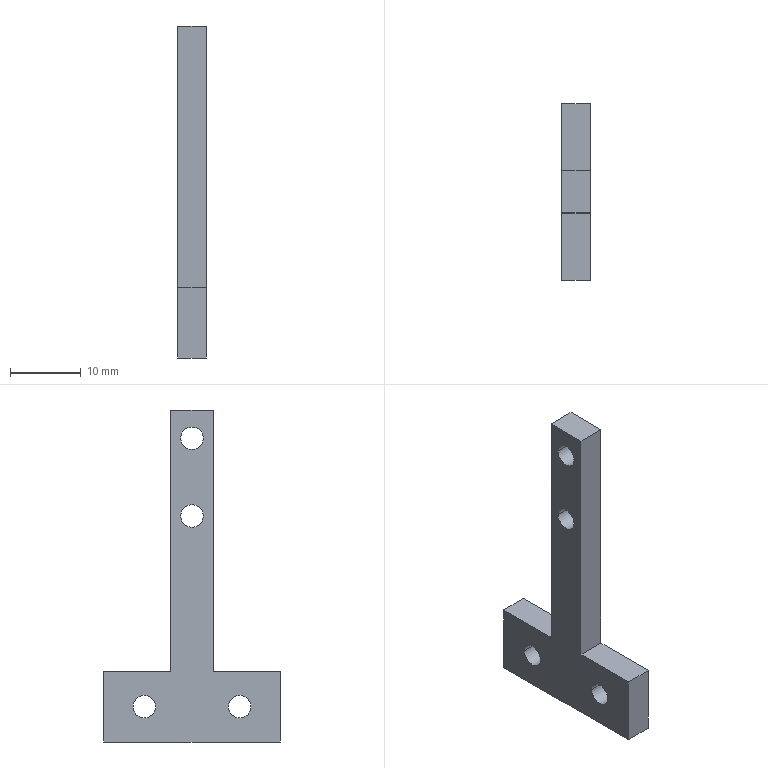Part | SolidWorks | features BaseBody 1 | 1 solid | 18 faces | box 4 x 25 x 47 mm | volume 1759 mm3 | plane 10 | cylinder 8 | commonest cylinder face diameters 3.2 x8
STEP:
#1=CARTESIAN_POINT('',(-908.131,394.397,204.732));
#2=VERTEX_POINT('',#1);
#3=CARTESIAN_POINT('',(-908.131,391.197,204.732));
#4=VERTEX_POINT('',#3);
#5=CARTESIAN_POINT('',(-908.131,392.797,204.732));
#6=DIRECTION('',(1.,0.,0.));
#7=DIRECTION('',(0.,1.,0.));
#8=AXIS2_PLACEMENT_3D('',#5,#6,#7);
#9=CIRCLE('',#8,1.6);
#10=EDGE_CURVE('',#2,#4,#9,.T.);
#11=ORIENTED_EDGE('',*,*,#10,.T.);
#12=CARTESIAN_POINT('',(-912.131,391.197,204.732));
#13=VERTEX_POINT('',#12);
#14=CARTESIAN_POINT('',(-912.131,391.197,204.732));
#15=DIRECTION('',(1.,0.,0.));
#16=VECTOR('',#15,1000.);
#17=LINE('',#14,#16);
#18=EDGE_CURVE('',#13,#4,#17,.T.);
#19=ORIENTED_EDGE('',*,*,#18,.F.);
#20=CARTESIAN_POINT('',(-912.131,394.397,204.732));
#21=VERTEX_POINT('',#20);
#22=CARTESIAN_POINT('',(-912.131,392.797,204.732));
#23=DIRECTION('',(-1.,0.,0.));
#24=DIRECTION('',(0.,-1.,0.));
#25=AXIS2_PLACEMENT_3D('',#22,#23,#24);
#26=CIRCLE('',#25,1.6);
#27=EDGE_CURVE('',#13,#21,#26,.T.);
#28=ORIENTED_EDGE('',*,*,#27,.T.);
#29=CARTESIAN_POINT('',(-908.131,394.397,204.732));
#30=DIRECTION('',(-1.,0.,0.));
#31=VECTOR('',#30,1000.);
#32=LINE('',#29,#31);
#33=EDGE_CURVE('',#2,#21,#32,.T.);
#34=ORIENTED_EDGE('',*,*,#33,.F.);
#35=EDGE_LOOP('',(#11,#19,#28,#34));
#36=FACE_OUTER_BOUND('',#35,.T.);
#37=CARTESIAN_POINT('',(-912.131,392.797,204.732));
#38=DIRECTION('',(1.,0.,0.));
#39=DIRECTION('',(0.,1.,0.));
#40=AXIS2_PLACEMENT_3D('',#37,#38,#39);
#41=CYLINDRICAL_SURFACE('',#40,1.6);
#42=ADVANCED_FACE('',(#36),#41,.F.);
#43=ORIENTED_EDGE('',*,*,#18,.T.);
#44=CARTESIAN_POINT('',(-908.131,392.797,204.732));
#45=DIRECTION('',(1.,0.,0.));
#46=DIRECTION('',(0.,-1.,0.));
#47=AXIS2_PLACEMENT_3D('',#44,#45,#46);
#48=CIRCLE('',#47,1.6);
#49=EDGE_CURVE('',#4,#2,#48,.T.);
#50=ORIENTED_EDGE('',*,*,#49,.T.);
#51=ORIENTED_EDGE('',*,*,#33,.T.);
#52=CARTESIAN_POINT('',(-912.131,392.797,204.732));
#53=DIRECTION('',(-1.,0.,0.));
#54=DIRECTION('',(0.,1.,0.));
#55=AXIS2_PLACEMENT_3D('',#52,#53,#54);
#56=CIRCLE('',#55,1.6);
#57=EDGE_CURVE('',#21,#13,#56,.T.);
#58=ORIENTED_EDGE('',*,*,#57,.T.);
#59=EDGE_LOOP('',(#43,#50,#51,#58));
#60=FACE_OUTER_BOUND('',#59,.T.);
#61=CARTESIAN_POINT('',(-912.131,392.797,204.732));
#62=DIRECTION('',(1.,0.,0.));
#63=DIRECTION('',(0.,1.,0.));
#64=AXIS2_PLACEMENT_3D('',#61,#62,#63);
#65=CYLINDRICAL_SURFACE('',#64,1.6);
#66=ADVANCED_FACE('',(#60),#65,.F.);
#67=CARTESIAN_POINT('',(-912.131,405.297,161.732));
#68=VERTEX_POINT('',#67);
#69=CARTESIAN_POINT('',(-912.131,405.297,171.732));
#70=VERTEX_POINT('',#69);
#71=CARTESIAN_POINT('',(-912.131,405.297,161.732));
#72=DIRECTION('',(0.,0.,1.));
#73=VECTOR('',#72,1000.);
#74=LINE('',#71,#73);
#75=EDGE_CURVE('',#68,#70,#74,.T.);
#76=ORIENTED_EDGE('',*,*,#75,.F.);
#77=CARTESIAN_POINT('',(-912.131,380.297,161.732));
#78=VERTEX_POINT('',#77);
#79=CARTESIAN_POINT('',(-912.131,380.297,161.732));
#80=DIRECTION('',(0.,1.,0.));
#81=VECTOR('',#80,1000.);
#82=LINE('',#79,#81);
#83=EDGE_CURVE('',#78,#68,#82,.T.);
#84=ORIENTED_EDGE('',*,*,#83,.F.);
#85=CARTESIAN_POINT('',(-912.131,380.297,171.732));
#86=VERTEX_POINT('',#85);
#87=CARTESIAN_POINT('',(-912.131,380.297,171.732));
#88=DIRECTION('',(0.,0.,-1.));
#89=VECTOR('',#88,1000.);
#90=LINE('',#87,#89);
#91=EDGE_CURVE('',#86,#78,#90,.T.);
#92=ORIENTED_EDGE('',*,*,#91,.F.);
#93=CARTESIAN_POINT('',(-912.131,389.797,171.732));
#94=VERTEX_POINT('',#93);
#95=CARTESIAN_POINT('',(-912.131,389.797,171.732));
#96=DIRECTION('',(0.,-1.,0.));
#97=VECTOR('',#96,1000.);
#98=LINE('',#95,#97);
#99=EDGE_CURVE('',#94,#86,#98,.T.);
#100=ORIENTED_EDGE('',*,*,#99,.F.);
#101=CARTESIAN_POINT('',(-912.131,389.797,208.732));
#102=VERTEX_POINT('',#101);
#103=CARTESIAN_POINT('',(-912.131,389.797,208.732));
#104=DIRECTION('',(0.,0.,-1.));
#105=VECTOR('',#104,1000.);
#106=LINE('',#103,#105);
#107=EDGE_CURVE('',#102,#94,#106,.T.);
#108=ORIENTED_EDGE('',*,*,#107,.F.);
#109=CARTESIAN_POINT('',(-912.131,395.797,208.732));
#110=VERTEX_POINT('',#109);
#111=CARTESIAN_POINT('',(-912.131,395.797,208.732));
#112=DIRECTION('',(0.,-1.,0.));
#113=VECTOR('',#112,1000.);
#114=LINE('',#111,#113);
#115=EDGE_CURVE('',#110,#102,#114,.T.);
#116=ORIENTED_EDGE('',*,*,#115,.F.);
#117=CARTESIAN_POINT('',(-912.131,395.797,171.732));
#118=VERTEX_POINT('',#117);
#119=CARTESIAN_POINT('',(-912.131,395.797,171.732));
#120=DIRECTION('',(0.,0.,1.));
#121=VECTOR('',#120,1000.);
#122=LINE('',#119,#121);
#123=EDGE_CURVE('',#118,#110,#122,.T.);
#124=ORIENTED_EDGE('',*,*,#123,.F.);
#125=CARTESIAN_POINT('',(-912.131,405.297,171.732));
#126=DIRECTION('',(0.,-1.,0.));
#127=VECTOR('',#126,1000.);
#128=LINE('',#125,#127);
#129=EDGE_CURVE('',#70,#118,#128,.T.);
#130=ORIENTED_EDGE('',*,*,#129,.F.);
#131=EDGE_LOOP('',(#76,#84,#92,#100,#108,#116,#124,#130));
#132=FACE_OUTER_BOUND('',#131,.T.);
#133=ORIENTED_EDGE('',*,*,#27,.F.);
#134=ORIENTED_EDGE('',*,*,#57,.F.);
#135=EDGE_LOOP('',(#133,#134));
#136=FACE_BOUND('',#135,.T.);
#137=CARTESIAN_POINT('',(-912.131,391.197,193.732));
#138=VERTEX_POINT('',#137);
#139=CARTESIAN_POINT('',(-912.131,394.397,193.732));
#140=VERTEX_POINT('',#139);
#141=CARTESIAN_POINT('',(-912.131,392.797,193.732));
#142=DIRECTION('',(-1.,0.,0.));
#143=DIRECTION('',(0.,-1.,0.));
#144=AXIS2_PLACEMENT_3D('',#141,#142,#143);
#145=CIRCLE('',#144,1.6);
#146=EDGE_CURVE('',#138,#140,#145,.T.);
#147=ORIENTED_EDGE('',*,*,#146,.F.);
#148=CARTESIAN_POINT('',(-912.131,392.797,193.732));
#149=DIRECTION('',(-1.,0.,0.));
#150=DIRECTION('',(0.,1.,0.));
#151=AXIS2_PLACEMENT_3D('',#148,#149,#150);
#152=CIRCLE('',#151,1.6);
#153=EDGE_CURVE('',#140,#138,#152,.T.);
#154=ORIENTED_EDGE('',*,*,#153,.F.);
#155=EDGE_LOOP('',(#147,#154));
#156=FACE_BOUND('',#155,.T.);
#157=CARTESIAN_POINT('',(-912.131,384.447,166.732));
#158=VERTEX_POINT('',#157);
#159=CARTESIAN_POINT('',(-912.131,387.647,166.732));
#160=VERTEX_POINT('',#159);
#161=CARTESIAN_POINT('',(-912.131,386.047,166.732));
#162=DIRECTION('',(-1.,0.,0.));
#163=DIRECTION('',(0.,-1.,0.));
#164=AXIS2_PLACEMENT_3D('',#161,#162,#163);
#165=CIRCLE('',#164,1.6);
#166=EDGE_CURVE('',#158,#160,#165,.T.);
#167=ORIENTED_EDGE('',*,*,#166,.F.);
#168=CARTESIAN_POINT('',(-912.131,386.047,166.732));
#169=DIRECTION('',(-1.,0.,0.));
#170=DIRECTION('',(0.,1.,0.));
#171=AXIS2_PLACEMENT_3D('',#168,#169,#170);
#172=CIRCLE('',#171,1.6);
#173=EDGE_CURVE('',#160,#158,#172,.T.);
#174=ORIENTED_EDGE('',*,*,#173,.F.);
#175=EDGE_LOOP('',(#167,#174));
#176=FACE_BOUND('',#175,.T.);
#177=CARTESIAN_POINT('',(-912.131,401.147,166.732));
#178=VERTEX_POINT('',#177);
#179=CARTESIAN_POINT('',(-912.131,397.947,166.732));
#180=VERTEX_POINT('',#179);
#181=CARTESIAN_POINT('',(-912.131,399.547,166.732));
#182=DIRECTION('',(-1.,0.,0.));
#183=DIRECTION('',(0.,1.,0.));
#184=AXIS2_PLACEMENT_3D('',#181,#182,#183);
#185=CIRCLE('',#184,1.6);
#186=EDGE_CURVE('',#178,#180,#185,.T.);
#187=ORIENTED_EDGE('',*,*,#186,.F.);
#188=CARTESIAN_POINT('',(-912.131,399.547,166.732));
#189=DIRECTION('',(-1.,0.,0.));
#190=DIRECTION('',(0.,-1.,0.));
#191=AXIS2_PLACEMENT_3D('',#188,#189,#190);
#192=CIRCLE('',#191,1.6);
#193=EDGE_CURVE('',#180,#178,#192,.T.);
#194=ORIENTED_EDGE('',*,*,#193,.F.);
#195=EDGE_LOOP('',(#187,#194));
#196=FACE_BOUND('',#195,.T.);
#197=CARTESIAN_POINT('',(-912.131,392.797,166.732));
#198=DIRECTION('',(-1.,0.,0.));
#199=DIRECTION('',(0.,-1.,0.));
#200=AXIS2_PLACEMENT_3D('',#197,#198,#199);
#201=PLANE('',#200);
#202=ADVANCED_FACE('',(#132,#136,#156,#176,#196),#201,.T.);
#203=ORIENTED_EDGE('',*,*,#129,.T.);
#204=CARTESIAN_POINT('',(-908.131,395.797,171.732));
#205=VERTEX_POINT('',#204);
#206=CARTESIAN_POINT('',(-912.131,395.797,171.732));
#207=DIRECTION('',(1.,0.,0.));
#208=VECTOR('',#207,1000.);
#209=LINE('',#206,#208);
#210=EDGE_CURVE('',#118,#205,#209,.T.);
#211=ORIENTED_EDGE('',*,*,#210,.T.);
#212=CARTESIAN_POINT('',(-908.131,405.297,171.732));
#213=VERTEX_POINT('',#212);
#214=CARTESIAN_POINT('',(-908.131,395.797,171.732));
#215=DIRECTION('',(0.,1.,0.));
#216=VECTOR('',#215,1000.);
#217=LINE('',#214,#216);
#218=EDGE_CURVE('',#205,#213,#217,.T.);
#219=ORIENTED_EDGE('',*,*,#218,.T.);
#220=CARTESIAN_POINT('',(-912.131,405.297,171.732));
#221=DIRECTION('',(1.,0.,0.));
#222=VECTOR('',#221,1000.);
#223=LINE('',#220,#222);
#224=EDGE_CURVE('',#70,#213,#223,.T.);
#225=ORIENTED_EDGE('',*,*,#224,.F.);
#226=EDGE_LOOP('',(#203,#211,#219,#225));
#227=FACE_OUTER_BOUND('',#226,.T.);
#228=CARTESIAN_POINT('',(-912.131,392.797,171.732));
#229=DIRECTION('',(0.,0.,-1.));
#230=DIRECTION('',(0.,1.,0.));
#231=AXIS2_PLACEMENT_3D('',#228,#229,#230);
#232=PLANE('',#231);
#233=ADVANCED_FACE('',(#227),#232,.F.);
#234=ORIENTED_EDGE('',*,*,#75,.T.);
#235=ORIENTED_EDGE('',*,*,#224,.T.);
#236=CARTESIAN_POINT('',(-908.131,405.297,161.732));
#237=VERTEX_POINT('',#236);
#238=CARTESIAN_POINT('',(-908.131,405.297,171.732));
#239=DIRECTION('',(0.,0.,-1.));
#240=VECTOR('',#239,1000.);
#241=LINE('',#238,#240);
#242=EDGE_CURVE('',#213,#237,#241,.T.);
#243=ORIENTED_EDGE('',*,*,#242,.T.);
#244=CARTESIAN_POINT('',(-912.131,405.297,161.732));
#245=DIRECTION('',(1.,0.,0.));
#246=VECTOR('',#245,1000.);
#247=LINE('',#244,#246);
#248=EDGE_CURVE('',#68,#237,#247,.T.);
#249=ORIENTED_EDGE('',*,*,#248,.F.);
#250=EDGE_LOOP('',(#234,#235,#243,#249));
#251=FACE_OUTER_BOUND('',#250,.T.);
#252=CARTESIAN_POINT('',(-912.131,405.297,166.732));
#253=DIRECTION('',(0.,1.,0.));
#254=DIRECTION('',(0.,0.,1.));
#255=AXIS2_PLACEMENT_3D('',#252,#253,#254);
#256=PLANE('',#255);
#257=ADVANCED_FACE('',(#251),#256,.T.);
#258=ORIENTED_EDGE('',*,*,#83,.T.);
#259=ORIENTED_EDGE('',*,*,#248,.T.);
#260=CARTESIAN_POINT('',(-908.131,380.297,161.732));
#261=VERTEX_POINT('',#260);
#262=CARTESIAN_POINT('',(-908.131,405.297,161.732));
#263=DIRECTION('',(0.,-1.,0.));
#264=VECTOR('',#263,1000.);
#265=LINE('',#262,#264);
#266=EDGE_CURVE('',#237,#261,#265,.T.);
#267=ORIENTED_EDGE('',*,*,#266,.T.);
#268=CARTESIAN_POINT('',(-912.131,380.297,161.732));
#269=DIRECTION('',(1.,0.,0.));
#270=VECTOR('',#269,1000.);
#271=LINE('',#268,#270);
#272=EDGE_CURVE('',#78,#261,#271,.T.);
#273=ORIENTED_EDGE('',*,*,#272,.F.);
#274=EDGE_LOOP('',(#258,#259,#267,#273));
#275=FACE_OUTER_BOUND('',#274,.T.);
#276=CARTESIAN_POINT('',(-912.131,392.797,161.732));
#277=DIRECTION('',(0.,0.,-1.));
#278=DIRECTION('',(0.,1.,0.));
#279=AXIS2_PLACEMENT_3D('',#276,#277,#278);
#280=PLANE('',#279);
#281=ADVANCED_FACE('',(#275),#280,.T.);
#282=ORIENTED_EDGE('',*,*,#91,.T.);
#283=ORIENTED_EDGE('',*,*,#272,.T.);
#284=CARTESIAN_POINT('',(-908.131,380.297,171.732));
#285=VERTEX_POINT('',#284);
#286=CARTESIAN_POINT('',(-908.131,380.297,161.732));
#287=DIRECTION('',(0.,0.,1.));
#288=VECTOR('',#287,1000.);
#289=LINE('',#286,#288);
#290=EDGE_CURVE('',#261,#285,#289,.T.);
#291=ORIENTED_EDGE('',*,*,#290,.T.);
#292=CARTESIAN_POINT('',(-912.131,380.297,171.732));
#293=DIRECTION('',(1.,0.,0.));
#294=VECTOR('',#293,1000.);
#295=LINE('',#292,#294);
#296=EDGE_CURVE('',#86,#285,#295,.T.);
#297=ORIENTED_EDGE('',*,*,#296,.F.);
#298=EDGE_LOOP('',(#282,#283,#291,#297));
#299=FACE_OUTER_BOUND('',#298,.T.);
#300=CARTESIAN_POINT('',(-912.131,380.297,166.732));
#301=DIRECTION('',(0.,1.,0.));
#302=DIRECTION('',(0.,0.,1.));
#303=AXIS2_PLACEMENT_3D('',#300,#301,#302);
#304=PLANE('',#303);
#305=ADVANCED_FACE('',(#299),#304,.F.);
#306=ORIENTED_EDGE('',*,*,#99,.T.);
#307=ORIENTED_EDGE('',*,*,#296,.T.);
#308=CARTESIAN_POINT('',(-908.131,389.797,171.732));
#309=VERTEX_POINT('',#308);
#310=CARTESIAN_POINT('',(-908.131,380.297,171.732));
#311=DIRECTION('',(0.,1.,0.));
#312=VECTOR('',#311,1000.);
#313=LINE('',#310,#312);
#314=EDGE_CURVE('',#285,#309,#313,.T.);
#315=ORIENTED_EDGE('',*,*,#314,.T.);
#316=CARTESIAN_POINT('',(-912.131,389.797,171.732));
#317=DIRECTION('',(1.,0.,0.));
#318=VECTOR('',#317,1000.);
#319=LINE('',#316,#318);
#320=EDGE_CURVE('',#94,#309,#319,.T.);
#321=ORIENTED_EDGE('',*,*,#320,.F.);
#322=EDGE_LOOP('',(#306,#307,#315,#321));
#323=FACE_OUTER_BOUND('',#322,.T.);
#324=CARTESIAN_POINT('',(-912.131,392.797,171.732));
#325=DIRECTION('',(0.,0.,-1.));
#326=DIRECTION('',(0.,1.,0.));
#327=AXIS2_PLACEMENT_3D('',#324,#325,#326);
#328=PLANE('',#327);
#329=ADVANCED_FACE('',(#323),#328,.F.);
#330=ORIENTED_EDGE('',*,*,#107,.T.);
#331=ORIENTED_EDGE('',*,*,#320,.T.);
#332=CARTESIAN_POINT('',(-908.131,389.797,208.732));
#333=VERTEX_POINT('',#332);
#334=CARTESIAN_POINT('',(-908.131,389.797,171.732));
#335=DIRECTION('',(0.,0.,1.));
#336=VECTOR('',#335,1000.);
#337=LINE('',#334,#336);
#338=EDGE_CURVE('',#309,#333,#337,.T.);
#339=ORIENTED_EDGE('',*,*,#338,.T.);
#340=CARTESIAN_POINT('',(-912.131,389.797,208.732));
#341=DIRECTION('',(1.,0.,0.));
#342=VECTOR('',#341,1000.);
#343=LINE('',#340,#342);
#344=EDGE_CURVE('',#102,#333,#343,.T.);
#345=ORIENTED_EDGE('',*,*,#344,.F.);
#346=EDGE_LOOP('',(#330,#331,#339,#345));
#347=FACE_OUTER_BOUND('',#346,.T.);
#348=CARTESIAN_POINT('',(-912.131,389.797,166.732));
#349=DIRECTION('',(0.,1.,0.));
#350=DIRECTION('',(0.,0.,1.));
#351=AXIS2_PLACEMENT_3D('',#348,#349,#350);
#352=PLANE('',#351);
#353=ADVANCED_FACE('',(#347),#352,.F.);
#354=ORIENTED_EDGE('',*,*,#115,.T.);
#355=ORIENTED_EDGE('',*,*,#344,.T.);
#356=CARTESIAN_POINT('',(-908.131,395.797,208.732));
#357=VERTEX_POINT('',#356);
#358=CARTESIAN_POINT('',(-908.131,389.797,208.732));
#359=DIRECTION('',(0.,1.,0.));
#360=VECTOR('',#359,1000.);
#361=LINE('',#358,#360);
#362=EDGE_CURVE('',#333,#357,#361,.T.);
#363=ORIENTED_EDGE('',*,*,#362,.T.);
#364=CARTESIAN_POINT('',(-908.131,395.797,208.732));
#365=DIRECTION('',(-1.,0.,0.));
#366=VECTOR('',#365,1000.);
#367=LINE('',#364,#366);
#368=EDGE_CURVE('',#357,#110,#367,.T.);
#369=ORIENTED_EDGE('',*,*,#368,.T.);
#370=EDGE_LOOP('',(#354,#355,#363,#369));
#371=FACE_OUTER_BOUND('',#370,.T.);
#372=CARTESIAN_POINT('',(-912.131,392.797,208.732));
#373=DIRECTION('',(0.,0.,1.));
#374=DIRECTION('',(-1.,0.,0.));
#375=AXIS2_PLACEMENT_3D('',#372,#373,#374);
#376=PLANE('',#375);
#377=ADVANCED_FACE('',(#371),#376,.T.);
#378=ORIENTED_EDGE('',*,*,#123,.T.);
#379=ORIENTED_EDGE('',*,*,#368,.F.);
#380=CARTESIAN_POINT('',(-908.131,395.797,171.732));
#381=DIRECTION('',(0.,0.,1.));
#382=VECTOR('',#381,1000.);
#383=LINE('',#380,#382);
#384=EDGE_CURVE('',#205,#357,#383,.T.);
#385=ORIENTED_EDGE('',*,*,#384,.F.);
#386=ORIENTED_EDGE('',*,*,#210,.F.);
#387=EDGE_LOOP('',(#378,#379,#385,#386));
#388=FACE_OUTER_BOUND('',#387,.T.);
#389=CARTESIAN_POINT('',(-912.131,395.797,166.732));
#390=DIRECTION('',(0.,1.,0.));
#391=DIRECTION('',(0.,0.,1.));
#392=AXIS2_PLACEMENT_3D('',#389,#390,#391);
#393=PLANE('',#392);
#394=ADVANCED_FACE('',(#388),#393,.T.);
#395=ORIENTED_EDGE('',*,*,#338,.F.);
#396=ORIENTED_EDGE('',*,*,#314,.F.);
#397=ORIENTED_EDGE('',*,*,#290,.F.);
#398=ORIENTED_EDGE('',*,*,#266,.F.);
#399=ORIENTED_EDGE('',*,*,#242,.F.);
#400=ORIENTED_EDGE('',*,*,#218,.F.);
#401=ORIENTED_EDGE('',*,*,#384,.T.);
#402=ORIENTED_EDGE('',*,*,#362,.F.);
#403=EDGE_LOOP('',(#395,#396,#397,#398,#399,#400,#401,#402));
#404=FACE_OUTER_BOUND('',#403,.T.);
#405=ORIENTED_EDGE('',*,*,#10,.F.);
#406=ORIENTED_EDGE('',*,*,#49,.F.);
#407=EDGE_LOOP('',(#405,#406));
#408=FACE_BOUND('',#407,.T.);
#409=CARTESIAN_POINT('',(-908.131,394.397,193.732));
#410=VERTEX_POINT('',#409);
#411=CARTESIAN_POINT('',(-908.131,391.197,193.732));
#412=VERTEX_POINT('',#411);
#413=CARTESIAN_POINT('',(-908.131,392.797,193.732));
#414=DIRECTION('',(1.,0.,0.));
#415=DIRECTION('',(0.,1.,0.));
#416=AXIS2_PLACEMENT_3D('',#413,#414,#415);
#417=CIRCLE('',#416,1.6);
#418=EDGE_CURVE('',#410,#412,#417,.T.);
#419=ORIENTED_EDGE('',*,*,#418,.F.);
#420=CARTESIAN_POINT('',(-908.131,392.797,193.732));
#421=DIRECTION('',(1.,0.,0.));
#422=DIRECTION('',(0.,-1.,0.));
#423=AXIS2_PLACEMENT_3D('',#420,#421,#422);
#424=CIRCLE('',#423,1.6);
#425=EDGE_CURVE('',#412,#410,#424,.T.);
#426=ORIENTED_EDGE('',*,*,#425,.F.);
#427=EDGE_LOOP('',(#419,#426));
#428=FACE_BOUND('',#427,.T.);
#429=CARTESIAN_POINT('',(-908.131,387.647,166.732));
#430=VERTEX_POINT('',#429);
#431=CARTESIAN_POINT('',(-908.131,384.447,166.732));
#432=VERTEX_POINT('',#431);
#433=CARTESIAN_POINT('',(-908.131,386.047,166.732));
#434=DIRECTION('',(1.,0.,0.));
#435=DIRECTION('',(0.,1.,0.));
#436=AXIS2_PLACEMENT_3D('',#433,#434,#435);
#437=CIRCLE('',#436,1.6);
#438=EDGE_CURVE('',#430,#432,#437,.T.);
#439=ORIENTED_EDGE('',*,*,#438,.F.);
#440=CARTESIAN_POINT('',(-908.131,386.047,166.732));
#441=DIRECTION('',(1.,0.,0.));
#442=DIRECTION('',(0.,-1.,0.));
#443=AXIS2_PLACEMENT_3D('',#440,#441,#442);
#444=CIRCLE('',#443,1.6);
#445=EDGE_CURVE('',#432,#430,#444,.T.);
#446=ORIENTED_EDGE('',*,*,#445,.F.);
#447=EDGE_LOOP('',(#439,#446));
#448=FACE_BOUND('',#447,.T.);
#449=CARTESIAN_POINT('',(-908.131,397.947,166.732));
#450=VERTEX_POINT('',#449);
#451=CARTESIAN_POINT('',(-908.131,401.147,166.732));
#452=VERTEX_POINT('',#451);
#453=CARTESIAN_POINT('',(-908.131,399.547,166.732));
#454=DIRECTION('',(1.,0.,0.));
#455=DIRECTION('',(0.,-1.,0.));
#456=AXIS2_PLACEMENT_3D('',#453,#454,#455);
#457=CIRCLE('',#456,1.6);
#458=EDGE_CURVE('',#450,#452,#457,.T.);
#459=ORIENTED_EDGE('',*,*,#458,.F.);
#460=CARTESIAN_POINT('',(-908.131,399.547,166.732));
#461=DIRECTION('',(1.,0.,0.));
#462=DIRECTION('',(0.,1.,0.));
#463=AXIS2_PLACEMENT_3D('',#460,#461,#462);
#464=CIRCLE('',#463,1.6);
#465=EDGE_CURVE('',#452,#450,#464,.T.);
#466=ORIENTED_EDGE('',*,*,#465,.F.);
#467=EDGE_LOOP('',(#459,#466));
#468=FACE_BOUND('',#467,.T.);
#469=CARTESIAN_POINT('',(-908.131,392.797,166.732));
#470=DIRECTION('',(-1.,0.,0.));
#471=DIRECTION('',(0.,-1.,0.));
#472=AXIS2_PLACEMENT_3D('',#469,#470,#471);
#473=PLANE('',#472);
#474=ADVANCED_FACE('',(#404,#408,#428,#448,#468),#473,.F.);
#475=CARTESIAN_POINT('',(-912.131,391.197,193.732));
#476=DIRECTION('',(1.,0.,0.));
#477=VECTOR('',#476,1000.);
#478=LINE('',#475,#477);
#479=EDGE_CURVE('',#138,#412,#478,.T.);
#480=ORIENTED_EDGE('',*,*,#479,.T.);
#481=ORIENTED_EDGE('',*,*,#425,.T.);
#482=CARTESIAN_POINT('',(-908.131,394.397,193.732));
#483=DIRECTION('',(-1.,0.,0.));
#484=VECTOR('',#483,1000.);
#485=LINE('',#482,#484);
#486=EDGE_CURVE('',#410,#140,#485,.T.);
#487=ORIENTED_EDGE('',*,*,#486,.T.);
#488=ORIENTED_EDGE('',*,*,#153,.T.);
#489=EDGE_LOOP('',(#480,#481,#487,#488));
#490=FACE_OUTER_BOUND('',#489,.T.);
#491=CARTESIAN_POINT('',(-912.131,392.797,193.732));
#492=DIRECTION('',(1.,0.,0.));
#493=DIRECTION('',(0.,1.,0.));
#494=AXIS2_PLACEMENT_3D('',#491,#492,#493);
#495=CYLINDRICAL_SURFACE('',#494,1.6);
#496=ADVANCED_FACE('',(#490),#495,.F.);
#497=ORIENTED_EDGE('',*,*,#418,.T.);
#498=ORIENTED_EDGE('',*,*,#479,.F.);
#499=ORIENTED_EDGE('',*,*,#146,.T.);
#500=ORIENTED_EDGE('',*,*,#486,.F.);
#501=EDGE_LOOP('',(#497,#498,#499,#500));
#502=FACE_OUTER_BOUND('',#501,.T.);
#503=CARTESIAN_POINT('',(-912.131,392.797,193.732));
#504=DIRECTION('',(1.,0.,0.));
#505=DIRECTION('',(0.,1.,0.));
#506=AXIS2_PLACEMENT_3D('',#503,#504,#505);
#507=CYLINDRICAL_SURFACE('',#506,1.6);
#508=ADVANCED_FACE('',(#502),#507,.F.);
#509=CARTESIAN_POINT('',(-912.131,384.447,166.732));
#510=DIRECTION('',(1.,0.,0.));
#511=VECTOR('',#510,1000.);
#512=LINE('',#509,#511);
#513=EDGE_CURVE('',#158,#432,#512,.T.);
#514=ORIENTED_EDGE('',*,*,#513,.T.);
#515=ORIENTED_EDGE('',*,*,#445,.T.);
#516=CARTESIAN_POINT('',(-908.131,387.647,166.732));
#517=DIRECTION('',(-1.,0.,0.));
#518=VECTOR('',#517,1000.);
#519=LINE('',#516,#518);
#520=EDGE_CURVE('',#430,#160,#519,.T.);
#521=ORIENTED_EDGE('',*,*,#520,.T.);
#522=ORIENTED_EDGE('',*,*,#173,.T.);
#523=EDGE_LOOP('',(#514,#515,#521,#522));
#524=FACE_OUTER_BOUND('',#523,.T.);
#525=CARTESIAN_POINT('',(-912.131,386.047,166.732));
#526=DIRECTION('',(1.,0.,0.));
#527=DIRECTION('',(0.,1.,0.));
#528=AXIS2_PLACEMENT_3D('',#525,#526,#527);
#529=CYLINDRICAL_SURFACE('',#528,1.6);
#530=ADVANCED_FACE('',(#524),#529,.F.);
#531=ORIENTED_EDGE('',*,*,#438,.T.);
#532=ORIENTED_EDGE('',*,*,#513,.F.);
#533=ORIENTED_EDGE('',*,*,#166,.T.);
#534=ORIENTED_EDGE('',*,*,#520,.F.);
#535=EDGE_LOOP('',(#531,#532,#533,#534));
#536=FACE_OUTER_BOUND('',#535,.T.);
#537=CARTESIAN_POINT('',(-912.131,386.047,166.732));
#538=DIRECTION('',(1.,0.,0.));
#539=DIRECTION('',(0.,1.,0.));
#540=AXIS2_PLACEMENT_3D('',#537,#538,#539);
#541=CYLINDRICAL_SURFACE('',#540,1.6);
#542=ADVANCED_FACE('',(#536),#541,.F.);
#543=ORIENTED_EDGE('',*,*,#465,.T.);
#544=CARTESIAN_POINT('',(-908.131,397.947,166.732));
#545=DIRECTION('',(-1.,0.,0.));
#546=VECTOR('',#545,1000.);
#547=LINE('',#544,#546);
#548=EDGE_CURVE('',#450,#180,#547,.T.);
#549=ORIENTED_EDGE('',*,*,#548,.T.);
#550=ORIENTED_EDGE('',*,*,#193,.T.);
#551=CARTESIAN_POINT('',(-912.131,401.147,166.732));
#552=DIRECTION('',(1.,0.,0.));
#553=VECTOR('',#552,1000.);
#554=LINE('',#551,#553);
#555=EDGE_CURVE('',#178,#452,#554,.T.);
#556=ORIENTED_EDGE('',*,*,#555,.T.);
#557=EDGE_LOOP('',(#543,#549,#550,#556));
#558=FACE_OUTER_BOUND('',#557,.T.);
#559=CARTESIAN_POINT('',(-912.131,399.547,166.732));
#560=DIRECTION('',(1.,0.,0.));
#561=DIRECTION('',(0.,1.,0.));
#562=AXIS2_PLACEMENT_3D('',#559,#560,#561);
#563=CYLINDRICAL_SURFACE('',#562,1.6);
#564=ADVANCED_FACE('',(#558),#563,.F.);
#565=ORIENTED_EDGE('',*,*,#548,.F.);
#566=ORIENTED_EDGE('',*,*,#458,.T.);
#567=ORIENTED_EDGE('',*,*,#555,.F.);
#568=ORIENTED_EDGE('',*,*,#186,.T.);
#569=EDGE_LOOP('',(#565,#566,#567,#568));
#570=FACE_OUTER_BOUND('',#569,.T.);
#571=CARTESIAN_POINT('',(-912.131,399.547,166.732));
#572=DIRECTION('',(1.,0.,0.));
#573=DIRECTION('',(0.,1.,0.));
#574=AXIS2_PLACEMENT_3D('',#571,#572,#573);
#575=CYLINDRICAL_SURFACE('',#574,1.6);
#576=ADVANCED_FACE('',(#570),#575,.F.);
#577=CLOSED_SHELL('',(#42,#66,#202,#233,#257,#281,#305,#329,#353,#377,#394,#474,#496,#508,#530,#542,#564,#576));
#578=MANIFOLD_SOLID_BREP('',#577);
#579=CARTESIAN_POINT('',(0.,0.,0.));
#580=DIRECTION('',(0.,0.,1.));
#581=DIRECTION('',(1.,0.,0.));
#582=AXIS2_PLACEMENT_3D('',#579,#580,#581);
#583=(LENGTH_UNIT()NAMED_UNIT(*)SI_UNIT(.MILLI.,.METRE.));
#584=UNCERTAINTY_MEASURE_WITH_UNIT(LENGTH_MEASURE(0.00001),#583,'','');
#585=(NAMED_UNIT(*)PLANE_ANGLE_UNIT()SI_UNIT($,.RADIAN.));
#586=(NAMED_UNIT(*)SI_UNIT($,.STERADIAN.)SOLID_ANGLE_UNIT());
#587=(GEOMETRIC_REPRESENTATION_CONTEXT(3)GLOBAL_UNCERTAINTY_ASSIGNED_CONTEXT((#584))GLOBAL_UNIT_ASSIGNED_CONTEXT((#583,#585,#586))REPRESENTATION_CONTEXT('',''));
#588=ADVANCED_BREP_SHAPE_REPRESENTATION('',(#578,#582),#587);